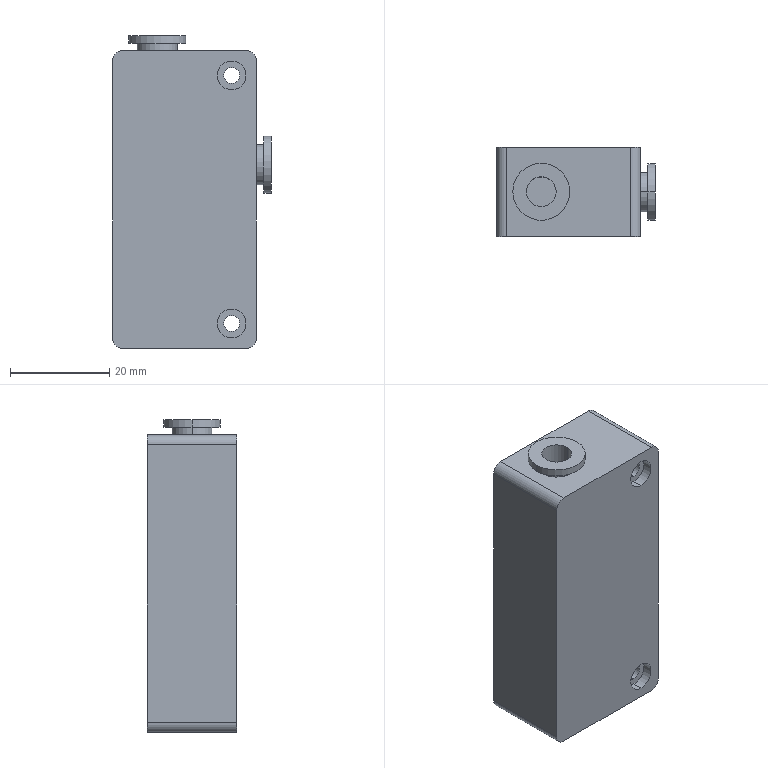Part | STEP file | ZH10BS_06_06_ZH10BS-06-06 | 1 solid | 44 faces | box 32 x 18 x 63 mm | volume 30323 mm3 | cylinder 28 | plane 16 | commonest cylinder face diameters 5.8 x8 3.2 x4 4 x4 6 x4 8 x4 11.5 x4
STEP:
#1=CARTESIAN_POINT('',(17.5,9.,10.));
#2=VERTEX_POINT('',#1);
#3=CARTESIAN_POINT('',(17.5,9.,4.));
#4=VERTEX_POINT('',#3);
#5=CARTESIAN_POINT('',(17.5,9.,7.));
#6=DIRECTION('',(1.,0.,0.));
#7=DIRECTION('',(0.,0.,1.));
#8=AXIS2_PLACEMENT_3D('',#5,#6,#7);
#9=CIRCLE('',#8,3.);
#10=EDGE_CURVE('',#2,#4,#9,.T.);
#11=ORIENTED_EDGE('',*,*,#10,.T.);
#12=CARTESIAN_POINT('',(0.5,9.,4.));
#13=VERTEX_POINT('',#12);
#14=CARTESIAN_POINT('',(17.51,9.,4.));
#15=DIRECTION('',(-1.,0.,0.));
#16=VECTOR('',#15,1000.);
#17=LINE('',#14,#16);
#18=EDGE_CURVE('',#4,#13,#17,.T.);
#19=ORIENTED_EDGE('',*,*,#18,.T.);
#20=CARTESIAN_POINT('',(0.5,9.,10.));
#21=VERTEX_POINT('',#20);
#22=CARTESIAN_POINT('',(0.5,9.,7.));
#23=DIRECTION('',(-1.,0.,0.));
#24=DIRECTION('',(0.,0.,1.));
#25=AXIS2_PLACEMENT_3D('',#22,#23,#24);
#26=CIRCLE('',#25,3.);
#27=EDGE_CURVE('',#13,#21,#26,.T.);
#28=ORIENTED_EDGE('',*,*,#27,.T.);
#29=CARTESIAN_POINT('',(17.51,9.,10.));
#30=DIRECTION('',(-1.,0.,0.));
#31=VECTOR('',#30,1000.);
#32=LINE('',#29,#31);
#33=EDGE_CURVE('',#2,#21,#32,.T.);
#34=ORIENTED_EDGE('',*,*,#33,.F.);
#35=EDGE_LOOP('',(#11,#19,#28,#34));
#36=FACE_OUTER_BOUND('',#35,.T.);
#37=CARTESIAN_POINT('',(17.51,9.,7.));
#38=DIRECTION('',(-1.,0.,0.));
#39=DIRECTION('',(0.,0.,1.));
#40=AXIS2_PLACEMENT_3D('',#37,#38,#39);
#41=CYLINDRICAL_SURFACE('',#40,3.);
#42=ADVANCED_FACE('',(#36),#41,.F.);
#43=CARTESIAN_POINT('',(16.,9.,1.25));
#44=VERTEX_POINT('',#43);
#45=CARTESIAN_POINT('',(16.,9.,12.75));
#46=VERTEX_POINT('',#45);
#47=CARTESIAN_POINT('',(16.,9.,7.));
#48=DIRECTION('',(1.,0.,0.));
#49=DIRECTION('',(0.,0.,-1.));
#50=AXIS2_PLACEMENT_3D('',#47,#48,#49);
#51=CIRCLE('',#50,5.75);
#52=EDGE_CURVE('',#44,#46,#51,.T.);
#53=ORIENTED_EDGE('',*,*,#52,.T.);
#54=CARTESIAN_POINT('',(17.5,9.,12.75));
#55=VERTEX_POINT('',#54);
#56=CARTESIAN_POINT('',(14.49,9.,12.75));
#57=DIRECTION('',(1.,0.,0.));
#58=VECTOR('',#57,1000.);
#59=LINE('',#56,#58);
#60=EDGE_CURVE('',#46,#55,#59,.T.);
#61=ORIENTED_EDGE('',*,*,#60,.T.);
#62=CARTESIAN_POINT('',(17.5,9.,1.25));
#63=VERTEX_POINT('',#62);
#64=CARTESIAN_POINT('',(17.5,9.,7.));
#65=DIRECTION('',(1.,0.,0.));
#66=DIRECTION('',(0.,0.,-1.));
#67=AXIS2_PLACEMENT_3D('',#64,#65,#66);
#68=CIRCLE('',#67,5.75);
#69=EDGE_CURVE('',#63,#55,#68,.T.);
#70=ORIENTED_EDGE('',*,*,#69,.F.);
#71=CARTESIAN_POINT('',(14.49,9.,1.25));
#72=DIRECTION('',(1.,0.,0.));
#73=VECTOR('',#72,1000.);
#74=LINE('',#71,#73);
#75=EDGE_CURVE('',#44,#63,#74,.T.);
#76=ORIENTED_EDGE('',*,*,#75,.F.);
#77=EDGE_LOOP('',(#53,#61,#70,#76));
#78=FACE_OUTER_BOUND('',#77,.T.);
#79=CARTESIAN_POINT('',(14.49,9.,7.));
#80=DIRECTION('',(1.,0.,0.));
#81=DIRECTION('',(0.,0.,-1.));
#82=AXIS2_PLACEMENT_3D('',#79,#80,#81);
#83=CYLINDRICAL_SURFACE('',#82,5.75);
#84=ADVANCED_FACE('',(#78),#83,.T.);
#85=CARTESIAN_POINT('',(14.5,9.,3.));
#86=VERTEX_POINT('',#85);
#87=CARTESIAN_POINT('',(14.5,9.,11.));
#88=VERTEX_POINT('',#87);
#89=CARTESIAN_POINT('',(14.5,9.,7.));
#90=DIRECTION('',(1.,0.,0.));
#91=DIRECTION('',(0.,0.,1.));
#92=AXIS2_PLACEMENT_3D('',#89,#90,#91);
#93=CIRCLE('',#92,4.);
#94=EDGE_CURVE('',#86,#88,#93,.T.);
#95=ORIENTED_EDGE('',*,*,#94,.T.);
#96=CARTESIAN_POINT('',(16.,9.,11.));
#97=VERTEX_POINT('',#96);
#98=CARTESIAN_POINT('',(14.49,9.,11.));
#99=DIRECTION('',(1.,0.,0.));
#100=VECTOR('',#99,1000.);
#101=LINE('',#98,#100);
#102=EDGE_CURVE('',#88,#97,#101,.T.);
#103=ORIENTED_EDGE('',*,*,#102,.T.);
#104=CARTESIAN_POINT('',(16.,9.,3.));
#105=VERTEX_POINT('',#104);
#106=CARTESIAN_POINT('',(16.,9.,7.));
#107=DIRECTION('',(1.,0.,0.));
#108=DIRECTION('',(0.,0.,-1.));
#109=AXIS2_PLACEMENT_3D('',#106,#107,#108);
#110=CIRCLE('',#109,4.);
#111=EDGE_CURVE('',#105,#97,#110,.T.);
#112=ORIENTED_EDGE('',*,*,#111,.F.);
#113=CARTESIAN_POINT('',(14.49,9.,3.));
#114=DIRECTION('',(1.,0.,0.));
#115=VECTOR('',#114,1000.);
#116=LINE('',#113,#115);
#117=EDGE_CURVE('',#86,#105,#116,.T.);
#118=ORIENTED_EDGE('',*,*,#117,.F.);
#119=EDGE_LOOP('',(#95,#103,#112,#118));
#120=FACE_OUTER_BOUND('',#119,.T.);
#121=CARTESIAN_POINT('',(14.49,9.,7.));
#122=DIRECTION('',(1.,0.,0.));
#123=DIRECTION('',(0.,0.,-1.));
#124=AXIS2_PLACEMENT_3D('',#121,#122,#123);
#125=CYLINDRICAL_SURFACE('',#124,4.);
#126=ADVANCED_FACE('',(#120),#125,.T.);
#127=CARTESIAN_POINT('',(-8.5,9.,16.));
#128=VERTEX_POINT('',#127);
#129=CARTESIAN_POINT('',(-2.5,9.,16.));
#130=VERTEX_POINT('',#129);
#131=CARTESIAN_POINT('',(-5.5,9.,16.));
#132=DIRECTION('',(0.,0.,1.));
#133=DIRECTION('',(1.,0.,0.));
#134=AXIS2_PLACEMENT_3D('',#131,#132,#133);
#135=CIRCLE('',#134,3.);
#136=EDGE_CURVE('',#128,#130,#135,.T.);
#137=ORIENTED_EDGE('',*,*,#136,.F.);
#138=CARTESIAN_POINT('',(-8.5,9.,33.));
#139=VERTEX_POINT('',#138);
#140=CARTESIAN_POINT('',(-8.5,9.,16.));
#141=DIRECTION('',(0.,0.,1.));
#142=VECTOR('',#141,1000.);
#143=LINE('',#140,#142);
#144=EDGE_CURVE('',#128,#139,#143,.T.);
#145=ORIENTED_EDGE('',*,*,#144,.T.);
#146=CARTESIAN_POINT('',(-2.5,9.,33.));
#147=VERTEX_POINT('',#146);
#148=CARTESIAN_POINT('',(-5.5,9.,33.));
#149=DIRECTION('',(0.,0.,1.));
#150=DIRECTION('',(-1.,0.,0.));
#151=AXIS2_PLACEMENT_3D('',#148,#149,#150);
#152=CIRCLE('',#151,3.);
#153=EDGE_CURVE('',#139,#147,#152,.T.);
#154=ORIENTED_EDGE('',*,*,#153,.T.);
#155=CARTESIAN_POINT('',(-2.5,9.,16.));
#156=DIRECTION('',(0.,0.,1.));
#157=VECTOR('',#156,1000.);
#158=LINE('',#155,#157);
#159=EDGE_CURVE('',#130,#147,#158,.T.);
#160=ORIENTED_EDGE('',*,*,#159,.F.);
#161=EDGE_LOOP('',(#137,#145,#154,#160));
#162=FACE_OUTER_BOUND('',#161,.T.);
#163=CARTESIAN_POINT('',(-5.5,9.,16.));
#164=DIRECTION('',(0.,0.,1.));
#165=DIRECTION('',(1.,0.,0.));
#166=AXIS2_PLACEMENT_3D('',#163,#164,#165);
#167=CYLINDRICAL_SURFACE('',#166,3.);
#168=ADVANCED_FACE('',(#162),#167,.F.);
#169=CARTESIAN_POINT('',(0.25,9.,31.5));
#170=VERTEX_POINT('',#169);
#171=CARTESIAN_POINT('',(-11.25,9.,31.5));
#172=VERTEX_POINT('',#171);
#173=CARTESIAN_POINT('',(-5.5,9.,31.5));
#174=DIRECTION('',(0.,0.,1.));
#175=DIRECTION('',(1.,0.,0.));
#176=AXIS2_PLACEMENT_3D('',#173,#174,#175);
#177=CIRCLE('',#176,5.75);
#178=EDGE_CURVE('',#170,#172,#177,.T.);
#179=ORIENTED_EDGE('',*,*,#178,.T.);
#180=CARTESIAN_POINT('',(-11.25,9.,33.));
#181=VERTEX_POINT('',#180);
#182=CARTESIAN_POINT('',(-11.25,9.,29.99));
#183=DIRECTION('',(0.,0.,1.));
#184=VECTOR('',#183,1000.);
#185=LINE('',#182,#184);
#186=EDGE_CURVE('',#172,#181,#185,.T.);
#187=ORIENTED_EDGE('',*,*,#186,.T.);
#188=CARTESIAN_POINT('',(0.25,9.,33.));
#189=VERTEX_POINT('',#188);
#190=CARTESIAN_POINT('',(-5.5,9.,33.));
#191=DIRECTION('',(0.,0.,1.));
#192=DIRECTION('',(1.,0.,0.));
#193=AXIS2_PLACEMENT_3D('',#190,#191,#192);
#194=CIRCLE('',#193,5.75);
#195=EDGE_CURVE('',#189,#181,#194,.T.);
#196=ORIENTED_EDGE('',*,*,#195,.F.);
#197=CARTESIAN_POINT('',(0.25,9.,29.99));
#198=DIRECTION('',(0.,0.,1.));
#199=VECTOR('',#198,1000.);
#200=LINE('',#197,#199);
#201=EDGE_CURVE('',#170,#189,#200,.T.);
#202=ORIENTED_EDGE('',*,*,#201,.F.);
#203=EDGE_LOOP('',(#179,#187,#196,#202));
#204=FACE_OUTER_BOUND('',#203,.T.);
#205=CARTESIAN_POINT('',(-5.5,9.,29.99));
#206=DIRECTION('',(0.,0.,1.));
#207=DIRECTION('',(1.,0.,0.));
#208=AXIS2_PLACEMENT_3D('',#205,#206,#207);
#209=CYLINDRICAL_SURFACE('',#208,5.75);
#210=ADVANCED_FACE('',(#204),#209,.T.);
#211=CARTESIAN_POINT('',(-1.5,9.,30.));
#212=VERTEX_POINT('',#211);
#213=CARTESIAN_POINT('',(-9.5,9.,30.));
#214=VERTEX_POINT('',#213);
#215=CARTESIAN_POINT('',(-5.5,9.,30.));
#216=DIRECTION('',(0.,0.,1.));
#217=DIRECTION('',(-1.,0.,0.));
#218=AXIS2_PLACEMENT_3D('',#215,#216,#217);
#219=CIRCLE('',#218,4.);
#220=EDGE_CURVE('',#212,#214,#219,.T.);
#221=ORIENTED_EDGE('',*,*,#220,.T.);
#222=CARTESIAN_POINT('',(-9.5,9.,31.5));
#223=VERTEX_POINT('',#222);
#224=CARTESIAN_POINT('',(-9.5,9.,29.99));
#225=DIRECTION('',(0.,0.,1.));
#226=VECTOR('',#225,1000.);
#227=LINE('',#224,#226);
#228=EDGE_CURVE('',#214,#223,#227,.T.);
#229=ORIENTED_EDGE('',*,*,#228,.T.);
#230=CARTESIAN_POINT('',(-1.5,9.,31.5));
#231=VERTEX_POINT('',#230);
#232=CARTESIAN_POINT('',(-5.5,9.,31.5));
#233=DIRECTION('',(0.,0.,1.));
#234=DIRECTION('',(1.,0.,0.));
#235=AXIS2_PLACEMENT_3D('',#232,#233,#234);
#236=CIRCLE('',#235,4.);
#237=EDGE_CURVE('',#231,#223,#236,.T.);
#238=ORIENTED_EDGE('',*,*,#237,.F.);
#239=CARTESIAN_POINT('',(-1.5,9.,29.99));
#240=DIRECTION('',(0.,0.,1.));
#241=VECTOR('',#240,1000.);
#242=LINE('',#239,#241);
#243=EDGE_CURVE('',#212,#231,#242,.T.);
#244=ORIENTED_EDGE('',*,*,#243,.F.);
#245=EDGE_LOOP('',(#221,#229,#238,#244));
#246=FACE_OUTER_BOUND('',#245,.T.);
#247=CARTESIAN_POINT('',(-5.5,9.,29.99));
#248=DIRECTION('',(0.,0.,1.));
#249=DIRECTION('',(1.,0.,0.));
#250=AXIS2_PLACEMENT_3D('',#247,#248,#249);
#251=CYLINDRICAL_SURFACE('',#250,4.);
#252=ADVANCED_FACE('',(#246),#251,.T.);
#253=CARTESIAN_POINT('',(9.5,2.,-26.6));
#254=VERTEX_POINT('',#253);
#255=CARTESIAN_POINT('',(9.5,2.,-23.4));
#256=VERTEX_POINT('',#255);
#257=CARTESIAN_POINT('',(9.5,2.,-25.));
#258=DIRECTION('',(0.,1.,0.));
#259=DIRECTION('',(0.,0.,1.));
#260=AXIS2_PLACEMENT_3D('',#257,#258,#259);
#261=CIRCLE('',#260,1.6);
#262=EDGE_CURVE('',#254,#256,#261,.T.);
#263=ORIENTED_EDGE('',*,*,#262,.F.);
#264=CARTESIAN_POINT('',(9.5,16.,-26.6));
#265=VERTEX_POINT('',#264);
#266=CARTESIAN_POINT('',(9.5,-2.,-26.6));
#267=DIRECTION('',(0.,1.,0.));
#268=VECTOR('',#267,1000.);
#269=LINE('',#266,#268);
#270=EDGE_CURVE('',#254,#265,#269,.T.);
#271=ORIENTED_EDGE('',*,*,#270,.T.);
#272=CARTESIAN_POINT('',(9.5,16.,-23.4));
#273=VERTEX_POINT('',#272);
#274=CARTESIAN_POINT('',(9.5,16.,-25.));
#275=DIRECTION('',(0.,1.,0.));
#276=DIRECTION('',(0.,0.,1.));
#277=AXIS2_PLACEMENT_3D('',#274,#275,#276);
#278=CIRCLE('',#277,1.6);
#279=EDGE_CURVE('',#265,#273,#278,.T.);
#280=ORIENTED_EDGE('',*,*,#279,.T.);
#281=CARTESIAN_POINT('',(9.5,-2.,-23.4));
#282=DIRECTION('',(0.,1.,0.));
#283=VECTOR('',#282,1000.);
#284=LINE('',#281,#283);
#285=EDGE_CURVE('',#256,#273,#284,.T.);
#286=ORIENTED_EDGE('',*,*,#285,.F.);
#287=EDGE_LOOP('',(#263,#271,#280,#286));
#288=FACE_OUTER_BOUND('',#287,.T.);
#289=CARTESIAN_POINT('',(9.5,-2.,-25.));
#290=DIRECTION('',(0.,1.,0.));
#291=DIRECTION('',(0.,0.,1.));
#292=AXIS2_PLACEMENT_3D('',#289,#290,#291);
#293=CYLINDRICAL_SURFACE('',#292,1.6);
#294=ADVANCED_FACE('',(#288),#293,.F.);
#295=CARTESIAN_POINT('',(9.5,16.,-27.9));
#296=VERTEX_POINT('',#295);
#297=CARTESIAN_POINT('',(9.5,16.,-22.1));
#298=VERTEX_POINT('',#297);
#299=CARTESIAN_POINT('',(9.5,16.,-25.));
#300=DIRECTION('',(0.,1.,0.));
#301=DIRECTION('',(0.,0.,1.));
#302=AXIS2_PLACEMENT_3D('',#299,#300,#301);
#303=CIRCLE('',#302,2.9);
#304=EDGE_CURVE('',#296,#298,#303,.T.);
#305=ORIENTED_EDGE('',*,*,#304,.F.);
#306=CARTESIAN_POINT('',(9.5,18.,-27.9));
#307=VERTEX_POINT('',#306);
#308=CARTESIAN_POINT('',(9.5,-2.,-27.9));
#309=DIRECTION('',(0.,1.,0.));
#310=VECTOR('',#309,1000.);
#311=LINE('',#308,#310);
#312=EDGE_CURVE('',#296,#307,#311,.T.);
#313=ORIENTED_EDGE('',*,*,#312,.T.);
#314=CARTESIAN_POINT('',(9.5,18.,-22.1));
#315=VERTEX_POINT('',#314);
#316=CARTESIAN_POINT('',(9.5,18.,-25.));
#317=DIRECTION('',(0.,-1.,0.));
#318=DIRECTION('',(0.,0.,1.));
#319=AXIS2_PLACEMENT_3D('',#316,#317,#318);
#320=CIRCLE('',#319,2.9);
#321=EDGE_CURVE('',#315,#307,#320,.T.);
#322=ORIENTED_EDGE('',*,*,#321,.F.);
#323=CARTESIAN_POINT('',(9.5,-2.,-22.1));
#324=DIRECTION('',(0.,1.,0.));
#325=VECTOR('',#324,1000.);
#326=LINE('',#323,#325);
#327=EDGE_CURVE('',#298,#315,#326,.T.);
#328=ORIENTED_EDGE('',*,*,#327,.F.);
#329=EDGE_LOOP('',(#305,#313,#322,#328));
#330=FACE_OUTER_BOUND('',#329,.T.);
#331=CARTESIAN_POINT('',(9.5,-2.,-25.));
#332=DIRECTION('',(0.,1.,0.));
#333=DIRECTION('',(0.,0.,1.));
#334=AXIS2_PLACEMENT_3D('',#331,#332,#333);
#335=CYLINDRICAL_SURFACE('',#334,2.9);
#336=ADVANCED_FACE('',(#330),#335,.F.);
#337=CARTESIAN_POINT('',(9.5,0.,-22.1));
#338=VERTEX_POINT('',#337);
#339=CARTESIAN_POINT('',(9.5,0.,-27.9));
#340=VERTEX_POINT('',#339);
#341=CARTESIAN_POINT('',(9.5,0.,-25.));
#342=DIRECTION('',(0.,-1.,0.));
#343=DIRECTION('',(0.,0.,1.));
#344=AXIS2_PLACEMENT_3D('',#341,#342,#343);
#345=CIRCLE('',#344,2.9);
#346=EDGE_CURVE('',#338,#340,#345,.T.);
#347=ORIENTED_EDGE('',*,*,#346,.T.);
#348=CARTESIAN_POINT('',(9.5,2.,-27.9));
#349=VERTEX_POINT('',#348);
#350=CARTESIAN_POINT('',(9.5,-2.,-27.9));
#351=DIRECTION('',(0.,1.,0.));
#352=VECTOR('',#351,1000.);
#353=LINE('',#350,#352);
#354=EDGE_CURVE('',#340,#349,#353,.T.);
#355=ORIENTED_EDGE('',*,*,#354,.T.);
#356=CARTESIAN_POINT('',(9.5,2.,-22.1));
#357=VERTEX_POINT('',#356);
#358=CARTESIAN_POINT('',(9.5,2.,-25.));
#359=DIRECTION('',(0.,1.,0.));
#360=DIRECTION('',(0.,0.,1.));
#361=AXIS2_PLACEMENT_3D('',#358,#359,#360);
#362=CIRCLE('',#361,2.9);
#363=EDGE_CURVE('',#349,#357,#362,.T.);
#364=ORIENTED_EDGE('',*,*,#363,.T.);
#365=CARTESIAN_POINT('',(9.5,-2.,-22.1));
#366=DIRECTION('',(0.,1.,0.));
#367=VECTOR('',#366,1000.);
#368=LINE('',#365,#367);
#369=EDGE_CURVE('',#338,#357,#368,.T.);
#370=ORIENTED_EDGE('',*,*,#369,.F.);
#371=EDGE_LOOP('',(#347,#355,#364,#370));
#372=FACE_OUTER_BOUND('',#371,.T.);
#373=CARTESIAN_POINT('',(9.5,-2.,-25.));
#374=DIRECTION('',(0.,1.,0.));
#375=DIRECTION('',(0.,0.,1.));
#376=AXIS2_PLACEMENT_3D('',#373,#374,#375);
#377=CYLINDRICAL_SURFACE('',#376,2.9);
#378=ADVANCED_FACE('',(#372),#377,.F.);
#379=CARTESIAN_POINT('',(9.5,2.,23.4));
#380=VERTEX_POINT('',#379);
#381=CARTESIAN_POINT('',(9.5,2.,26.6));
#382=VERTEX_POINT('',#381);
#383=CARTESIAN_POINT('',(9.5,2.,25.));
#384=DIRECTION('',(0.,1.,0.));
#385=DIRECTION('',(0.,0.,1.));
#386=AXIS2_PLACEMENT_3D('',#383,#384,#385);
#387=CIRCLE('',#386,1.6);
#388=EDGE_CURVE('',#380,#382,#387,.T.);
#389=ORIENTED_EDGE('',*,*,#388,.F.);
#390=CARTESIAN_POINT('',(9.5,16.,23.4));
#391=VERTEX_POINT('',#390);
#392=CARTESIAN_POINT('',(9.5,-2.,23.4));
#393=DIRECTION('',(0.,1.,0.));
#394=VECTOR('',#393,1000.);
#395=LINE('',#392,#394);
#396=EDGE_CURVE('',#380,#391,#395,.T.);
#397=ORIENTED_EDGE('',*,*,#396,.T.);
#398=CARTESIAN_POINT('',(9.5,16.,26.6));
#399=VERTEX_POINT('',#398);
#400=CARTESIAN_POINT('',(9.5,16.,25.));
#401=DIRECTION('',(0.,1.,0.));
#402=DIRECTION('',(0.,0.,1.));
#403=AXIS2_PLACEMENT_3D('',#400,#401,#402);
#404=CIRCLE('',#403,1.6);
#405=EDGE_CURVE('',#391,#399,#404,.T.);
#406=ORIENTED_EDGE('',*,*,#405,.T.);
#407=CARTESIAN_POINT('',(9.5,-2.,26.6));
#408=DIRECTION('',(0.,1.,0.));
#409=VECTOR('',#408,1000.);
#410=LINE('',#407,#409);
#411=EDGE_CURVE('',#382,#399,#410,.T.);
#412=ORIENTED_EDGE('',*,*,#411,.F.);
#413=EDGE_LOOP('',(#389,#397,#406,#412));
#414=FACE_OUTER_BOUND('',#413,.T.);
#415=CARTESIAN_POINT('',(9.5,-2.,25.));
#416=DIRECTION('',(0.,1.,0.));
#417=DIRECTION('',(0.,0.,1.));
#418=AXIS2_PLACEMENT_3D('',#415,#416,#417);
#419=CYLINDRICAL_SURFACE('',#418,1.6);
#420=ADVANCED_FACE('',(#414),#419,.F.);
#421=CARTESIAN_POINT('',(9.5,16.,22.1));
#422=VERTEX_POINT('',#421);
#423=CARTESIAN_POINT('',(9.5,16.,27.9));
#424=VERTEX_POINT('',#423);
#425=CARTESIAN_POINT('',(9.5,16.,25.));
#426=DIRECTION('',(0.,1.,0.));
#427=DIRECTION('',(0.,0.,1.));
#428=AXIS2_PLACEMENT_3D('',#425,#426,#427);
#429=CIRCLE('',#428,2.9);
#430=EDGE_CURVE('',#422,#424,#429,.T.);
#431=ORIENTED_EDGE('',*,*,#430,.F.);
#432=CARTESIAN_POINT('',(9.5,18.,22.1));
#433=VERTEX_POINT('',#432);
#434=CARTESIAN_POINT('',(9.5,-2.,22.1));
#435=DIRECTION('',(0.,1.,0.));
#436=VECTOR('',#435,1000.);
#437=LINE('',#434,#436);
#438=EDGE_CURVE('',#422,#433,#437,.T.);
#439=ORIENTED_EDGE('',*,*,#438,.T.);
#440=CARTESIAN_POINT('',(9.5,18.,27.9));
#441=VERTEX_POINT('',#440);
#442=CARTESIAN_POINT('',(9.5,18.,25.));
#443=DIRECTION('',(0.,-1.,0.));
#444=DIRECTION('',(0.,0.,1.));
#445=AXIS2_PLACEMENT_3D('',#442,#443,#444);
#446=CIRCLE('',#445,2.9);
#447=EDGE_CURVE('',#441,#433,#446,.T.);
#448=ORIENTED_EDGE('',*,*,#447,.F.);
#449=CARTESIAN_POINT('',(9.5,-2.,27.9));
#450=DIRECTION('',(0.,1.,0.));
#451=VECTOR('',#450,1000.);
#452=LINE('',#449,#451);
#453=EDGE_CURVE('',#424,#441,#452,.T.);
#454=ORIENTED_EDGE('',*,*,#453,.F.);
#455=EDGE_LOOP('',(#431,#439,#448,#454));
#456=FACE_OUTER_BOUND('',#455,.T.);
#457=CARTESIAN_POINT('',(9.5,-2.,25.));
#458=DIRECTION('',(0.,1.,0.));
#459=DIRECTION('',(0.,0.,1.));
#460=AXIS2_PLACEMENT_3D('',#457,#458,#459);
#461=CYLINDRICAL_SURFACE('',#460,2.9);
#462=ADVANCED_FACE('',(#456),#461,.F.);
#463=CARTESIAN_POINT('',(9.5,0.,27.9));
#464=VERTEX_POINT('',#463);
#465=CARTESIAN_POINT('',(9.5,0.,22.1));
#466=VERTEX_POINT('',#465);
#467=CARTESIAN_POINT('',(9.5,0.,25.));
#468=DIRECTION('',(0.,-1.,0.));
#469=DIRECTION('',(0.,0.,1.));
#470=AXIS2_PLACEMENT_3D('',#467,#468,#469);
#471=CIRCLE('',#470,2.9);
#472=EDGE_CURVE('',#464,#466,#471,.T.);
#473=ORIENTED_EDGE('',*,*,#472,.T.);
#474=CARTESIAN_POINT('',(9.5,2.,22.1));
#475=VERTEX_POINT('',#474);
#476=CARTESIAN_POINT('',(9.5,-2.,22.1));
#477=DIRECTION('',(0.,1.,0.));
#478=VECTOR('',#477,1000.);
#479=LINE('',#476,#478);
#480=EDGE_CURVE('',#466,#475,#479,.T.);
#481=ORIENTED_EDGE('',*,*,#480,.T.);
#482=CARTESIAN_POINT('',(9.5,2.,27.9));
#483=VERTEX_POINT('',#482);
#484=CARTESIAN_POINT('',(9.5,2.,25.));
#485=DIRECTION('',(0.,1.,0.));
#486=DIRECTION('',(0.,0.,1.));
#487=AXIS2_PLACEMENT_3D('',#484,#485,#486);
#488=CIRCLE('',#487,2.9);
#489=EDGE_CURVE('',#475,#483,#488,.T.);
#490=ORIENTED_EDGE('',*,*,#489,.T.);
#491=CARTESIAN_POINT('',(9.5,-2.,27.9));
#492=DIRECTION('',(0.,1.,0.));
#493=VECTOR('',#492,1000.);
#494=LINE('',#491,#493);
#495=EDGE_CURVE('',#464,#483,#494,.T.);
#496=ORIENTED_EDGE('',*,*,#495,.F.);
#497=EDGE_LOOP('',(#473,#481,#490,#496));
#498=FACE_OUTER_BOUND('',#497,.T.);
#499=CARTESIAN_POINT('',(9.5,-2.,25.));
#500=DIRECTION('',(0.,1.,0.));
#501=DIRECTION('',(0.,0.,1.));
#502=AXIS2_PLACEMENT_3D('',#499,#500,#501);
#503=CYLINDRICAL_SURFACE('',#502,2.9);
#504=ADVANCED_FACE('',(#498),#503,.F.);
#505=ORIENTED_EDGE('',*,*,#69,.T.);
#506=CARTESIAN_POINT('',(17.5,9.,7.));
#507=DIRECTION('',(1.,0.,0.));
#508=DIRECTION('',(0.,0.,-1.));
#509=AXIS2_PLACEMENT_3D('',#506,#507,#508);
#510=CIRCLE('',#509,5.75);
#511=EDGE_CURVE('',#55,#63,#510,.T.);
#512=ORIENTED_EDGE('',*,*,#511,.T.);
#513=EDGE_LOOP('',(#505,#512));
#514=FACE_OUTER_BOUND('',#513,.T.);
#515=ORIENTED_EDGE('',*,*,#10,.F.);
#516=CARTESIAN_POINT('',(17.5,9.,7.));
#517=DIRECTION('',(1.,0.,0.));
#518=DIRECTION('',(0.,0.,1.));
#519=AXIS2_PLACEMENT_3D('',#516,#517,#518);
#520=CIRCLE('',#519,3.);
#521=EDGE_CURVE('',#4,#2,#520,.T.);
#522=ORIENTED_EDGE('',*,*,#521,.F.);
#523=EDGE_LOOP('',(#515,#522));
#524=FACE_BOUND('',#523,.T.);
#525=CARTESIAN_POINT('',(17.5,9.,7.));
#526=DIRECTION('',(-1.,0.,0.));
#527=DIRECTION('',(0.,0.,1.));
#528=AXIS2_PLACEMENT_3D('',#525,#526,#527);
#529=PLANE('',#528);
#530=ADVANCED_FACE('',(#514,#524),#529,.F.);
#531=CARTESIAN_POINT('',(14.5,0.,28.));
#532=VERTEX_POINT('',#531);
#533=CARTESIAN_POINT('',(14.5,0.,-28.));
#534=VERTEX_POINT('',#533);
#535=CARTESIAN_POINT('',(14.5,0.,28.));
#536=DIRECTION('',(0.,0.,-1.));
#537=VECTOR('',#536,1000.);
#538=LINE('',#535,#537);
#539=EDGE_CURVE('',#532,#534,#538,.T.);
#540=ORIENTED_EDGE('',*,*,#539,.T.);
#541=CARTESIAN_POINT('',(14.5,18.,-28.));
#542=VERTEX_POINT('',#541);
#543=CARTESIAN_POINT('',(14.5,18.,-28.));
#544=DIRECTION('',(0.,-1.,0.));
#545=VECTOR('',#544,1000.);
#546=LINE('',#543,#545);
#547=EDGE_CURVE('',#542,#534,#546,.T.);
#548=ORIENTED_EDGE('',*,*,#547,.F.);
#549=CARTESIAN_POINT('',(14.5,18.,28.));
#550=VERTEX_POINT('',#549);
#551=CARTESIAN_POINT('',(14.5,18.,28.));
#552=DIRECTION('',(0.,0.,-1.));
#553=VECTOR('',#552,1000.);
#554=LINE('',#551,#553);
#555=EDGE_CURVE('',#550,#542,#554,.T.);
#556=ORIENTED_EDGE('',*,*,#555,.F.);
#557=CARTESIAN_POINT('',(14.5,18.,28.));
#558=DIRECTION('',(0.,-1.,0.));
#559=VECTOR('',#558,1000.);
#560=LINE('',#557,#559);
#561=EDGE_CURVE('',#550,#532,#560,.T.);
#562=ORIENTED_EDGE('',*,*,#561,.T.);
#563=EDGE_LOOP('',(#540,#548,#556,#562));
#564=FACE_OUTER_BOUND('',#563,.T.);
#565=ORIENTED_EDGE('',*,*,#94,.F.);
#566=CARTESIAN_POINT('',(14.5,9.,7.));
#567=DIRECTION('',(1.,0.,0.));
#568=DIRECTION('',(0.,0.,1.));
#569=AXIS2_PLACEMENT_3D('',#566,#567,#568);
#570=CIRCLE('',#569,4.);
#571=EDGE_CURVE('',#88,#86,#570,.T.);
#572=ORIENTED_EDGE('',*,*,#571,.F.);
#573=EDGE_LOOP('',(#565,#572));
#574=FACE_BOUND('',#573,.T.);
#575=CARTESIAN_POINT('',(14.5,18.,28.));
#576=DIRECTION('',(-1.,0.,0.));
#577=DIRECTION('',(0.,0.,1.));
#578=AXIS2_PLACEMENT_3D('',#575,#576,#577);
#579=PLANE('',#578);
#580=ADVANCED_FACE('',(#564,#574),#579,.F.);
#581=ORIENTED_EDGE('',*,*,#195,.T.);
#582=CARTESIAN_POINT('',(-5.5,9.,33.));
#583=DIRECTION('',(0.,0.,1.));
#584=DIRECTION('',(1.,0.,0.));
#585=AXIS2_PLACEMENT_3D('',#582,#583,#584);
#586=CIRCLE('',#585,5.75);
#587=EDGE_CURVE('',#181,#189,#586,.T.);
#588=ORIENTED_EDGE('',*,*,#587,.T.);
#589=EDGE_LOOP('',(#581,#588));
#590=FACE_OUTER_BOUND('',#589,.T.);
#591=CARTESIAN_POINT('',(-5.5,9.,33.));
#592=DIRECTION('',(0.,0.,1.));
#593=DIRECTION('',(-1.,0.,0.));
#594=AXIS2_PLACEMENT_3D('',#591,#592,#593);
#595=CIRCLE('',#594,3.);
#596=EDGE_CURVE('',#147,#139,#595,.T.);
#597=ORIENTED_EDGE('',*,*,#596,.F.);
#598=ORIENTED_EDGE('',*,*,#153,.F.);
#599=EDGE_LOOP('',(#597,#598));
#600=FACE_BOUND('',#599,.T.);
#601=CARTESIAN_POINT('',(-5.5,9.,33.));
#602=DIRECTION('',(0.,0.,-1.));
#603=DIRECTION('',(-1.,0.,0.));
#604=AXIS2_PLACEMENT_3D('',#601,#602,#603);
#605=PLANE('',#604);
#606=ADVANCED_FACE('',(#590,#600),#605,.F.);
#607=CARTESIAN_POINT('',(-12.5,0.,30.));
#608=VERTEX_POINT('',#607);
#609=CARTESIAN_POINT('',(12.5,0.,30.));
#610=VERTEX_POINT('',#609);
#611=CARTESIAN_POINT('',(-12.5,0.,30.));
#612=DIRECTION('',(1.,0.,0.));
#613=VECTOR('',#612,1000.);
#614=LINE('',#611,#613);
#615=EDGE_CURVE('',#608,#610,#614,.T.);
#616=ORIENTED_EDGE('',*,*,#615,.T.);
#617=CARTESIAN_POINT('',(12.5,18.,30.));
#618=VERTEX_POINT('',#617);
#619=CARTESIAN_POINT('',(12.5,18.,30.));
#620=DIRECTION('',(0.,-1.,0.));
#621=VECTOR('',#620,1000.);
#622=LINE('',#619,#621);
#623=EDGE_CURVE('',#618,#610,#622,.T.);
#624=ORIENTED_EDGE('',*,*,#623,.F.);
#625=CARTESIAN_POINT('',(-12.5,18.,30.));
#626=VERTEX_POINT('',#625);
#627=CARTESIAN_POINT('',(-12.5,18.,30.));
#628=DIRECTION('',(1.,0.,0.));
#629=VECTOR('',#628,1000.);
#630=LINE('',#627,#629);
#631=EDGE_CURVE('',#626,#618,#630,.T.);
#632=ORIENTED_EDGE('',*,*,#631,.F.);
#633=CARTESIAN_POINT('',(-12.5,18.,30.));
#634=DIRECTION('',(0.,-1.,0.));
#635=VECTOR('',#634,1000.);
#636=LINE('',#633,#635);
#637=EDGE_CURVE('',#626,#608,#636,.T.);
#638=ORIENTED_EDGE('',*,*,#637,.T.);
#639=EDGE_LOOP('',(#616,#624,#632,#638));
#640=FACE_OUTER_BOUND('',#639,.T.);
#641=ORIENTED_EDGE('',*,*,#220,.F.);
#642=CARTESIAN_POINT('',(-5.5,9.,30.));
#643=DIRECTION('',(0.,0.,1.));
#644=DIRECTION('',(-1.,0.,0.));
#645=AXIS2_PLACEMENT_3D('',#642,#643,#644);
#646=CIRCLE('',#645,4.);
#647=EDGE_CURVE('',#214,#212,#646,.T.);
#648=ORIENTED_EDGE('',*,*,#647,.F.);
#649=EDGE_LOOP('',(#641,#648));
#650=FACE_BOUND('',#649,.T.);
#651=CARTESIAN_POINT('',(-12.5,18.,30.));
#652=DIRECTION('',(0.,0.,-1.));
#653=DIRECTION('',(-1.,0.,0.));
#654=AXIS2_PLACEMENT_3D('',#651,#652,#653);
#655=PLANE('',#654);
#656=ADVANCED_FACE('',(#640,#650),#655,.F.);
#657=ORIENTED_EDGE('',*,*,#447,.T.);
#658=CARTESIAN_POINT('',(9.5,18.,25.));
#659=DIRECTION('',(0.,-1.,0.));
#660=DIRECTION('',(0.,0.,1.));
#661=AXIS2_PLACEMENT_3D('',#658,#659,#660);
#662=CIRCLE('',#661,2.9);
#663=EDGE_CURVE('',#433,#441,#662,.T.);
#664=ORIENTED_EDGE('',*,*,#663,.T.);
#665=EDGE_LOOP('',(#657,#664));
#666=FACE_BOUND('',#665,.T.);
#667=CARTESIAN_POINT('',(-14.5,18.,28.));
#668=VERTEX_POINT('',#667);
#669=CARTESIAN_POINT('',(-12.5,18.,28.));
#670=DIRECTION('',(0.,1.,0.));
#671=DIRECTION('',(0.,0.,1.));
#672=AXIS2_PLACEMENT_3D('',#669,#670,#671);
#673=CIRCLE('',#672,2.);
#674=EDGE_CURVE('',#668,#626,#673,.T.);
#675=ORIENTED_EDGE('',*,*,#674,.T.);
#676=ORIENTED_EDGE('',*,*,#631,.T.);
#677=CARTESIAN_POINT('',(12.5,18.,28.));
#678=DIRECTION('',(0.,1.,0.));
#679=DIRECTION('',(0.,0.,1.));
#680=AXIS2_PLACEMENT_3D('',#677,#678,#679);
#681=CIRCLE('',#680,2.);
#682=EDGE_CURVE('',#618,#550,#681,.T.);
#683=ORIENTED_EDGE('',*,*,#682,.T.);
#684=ORIENTED_EDGE('',*,*,#555,.T.);
#685=CARTESIAN_POINT('',(12.5,18.,-30.));
#686=VERTEX_POINT('',#685);
#687=CARTESIAN_POINT('',(12.5,18.,-28.));
#688=DIRECTION('',(0.,1.,0.));
#689=DIRECTION('',(0.,0.,1.));
#690=AXIS2_PLACEMENT_3D('',#687,#688,#689);
#691=CIRCLE('',#690,2.);
#692=EDGE_CURVE('',#542,#686,#691,.T.);
#693=ORIENTED_EDGE('',*,*,#692,.T.);
#694=CARTESIAN_POINT('',(-12.5,18.,-30.));
#695=VERTEX_POINT('',#694);
#696=CARTESIAN_POINT('',(12.5,18.,-30.));
#697=DIRECTION('',(-1.,0.,0.));
#698=VECTOR('',#697,1000.);
#699=LINE('',#696,#698);
#700=EDGE_CURVE('',#686,#695,#699,.T.);
#701=ORIENTED_EDGE('',*,*,#700,.T.);
#702=CARTESIAN_POINT('',(-14.5,18.,-28.));
#703=VERTEX_POINT('',#702);
#704=CARTESIAN_POINT('',(-12.5,18.,-28.));
#705=DIRECTION('',(0.,1.,0.));
#706=DIRECTION('',(0.,0.,1.));
#707=AXIS2_PLACEMENT_3D('',#704,#705,#706);
#708=CIRCLE('',#707,2.);
#709=EDGE_CURVE('',#695,#703,#708,.T.);
#710=ORIENTED_EDGE('',*,*,#709,.T.);
#711=CARTESIAN_POINT('',(-14.5,18.,-28.));
#712=DIRECTION('',(0.,0.,1.));
#713=VECTOR('',#712,1000.);
#714=LINE('',#711,#713);
#715=EDGE_CURVE('',#703,#668,#714,.T.);
#716=ORIENTED_EDGE('',*,*,#715,.T.);
#717=EDGE_LOOP('',(#675,#676,#683,#684,#693,#701,#710,#716));
#718=FACE_OUTER_BOUND('',#717,.T.);
#719=ORIENTED_EDGE('',*,*,#321,.T.);
#720=CARTESIAN_POINT('',(9.5,18.,-25.));
#721=DIRECTION('',(0.,-1.,0.));
#722=DIRECTION('',(0.,0.,1.));
#723=AXIS2_PLACEMENT_3D('',#720,#721,#722);
#724=CIRCLE('',#723,2.9);
#725=EDGE_CURVE('',#307,#315,#724,.T.);
#726=ORIENTED_EDGE('',*,*,#725,.T.);
#727=EDGE_LOOP('',(#719,#726));
#728=FACE_BOUND('',#727,.T.);
#729=CARTESIAN_POINT('',(-12.5,18.,28.));
#730=DIRECTION('',(0.,1.,0.));
#731=DIRECTION('',(0.,0.,1.));
#732=AXIS2_PLACEMENT_3D('',#729,#730,#731);
#733=PLANE('',#732);
#734=ADVANCED_FACE('',(#666,#718,#728),#733,.T.);
#735=ORIENTED_EDGE('',*,*,#472,.F.);
#736=CARTESIAN_POINT('',(9.5,0.,25.));
#737=DIRECTION('',(0.,-1.,0.));
#738=DIRECTION('',(0.,0.,1.));
#739=AXIS2_PLACEMENT_3D('',#736,#737,#738);
#740=CIRCLE('',#739,2.9);
#741=EDGE_CURVE('',#466,#464,#740,.T.);
#742=ORIENTED_EDGE('',*,*,#741,.F.);
#743=EDGE_LOOP('',(#735,#742));
#744=FACE_BOUND('',#743,.T.);
#745=CARTESIAN_POINT('',(-14.5,0.,28.));
#746=VERTEX_POINT('',#745);
#747=CARTESIAN_POINT('',(-12.5,0.,28.));
#748=DIRECTION('',(0.,1.,0.));
#749=DIRECTION('',(0.,0.,1.));
#750=AXIS2_PLACEMENT_3D('',#747,#748,#749);
#751=CIRCLE('',#750,2.);
#752=EDGE_CURVE('',#746,#608,#751,.T.);
#753=ORIENTED_EDGE('',*,*,#752,.F.);
#754=CARTESIAN_POINT('',(-14.5,0.,-28.));
#755=VERTEX_POINT('',#754);
#756=CARTESIAN_POINT('',(-14.5,0.,-28.));
#757=DIRECTION('',(0.,0.,1.));
#758=VECTOR('',#757,1000.);
#759=LINE('',#756,#758);
#760=EDGE_CURVE('',#755,#746,#759,.T.);
#761=ORIENTED_EDGE('',*,*,#760,.F.);
#762=CARTESIAN_POINT('',(-12.5,0.,-30.));
#763=VERTEX_POINT('',#762);
#764=CARTESIAN_POINT('',(-12.5,0.,-28.));
#765=DIRECTION('',(0.,1.,0.));
#766=DIRECTION('',(0.,0.,1.));
#767=AXIS2_PLACEMENT_3D('',#764,#765,#766);
#768=CIRCLE('',#767,2.);
#769=EDGE_CURVE('',#763,#755,#768,.T.);
#770=ORIENTED_EDGE('',*,*,#769,.F.);
#771=CARTESIAN_POINT('',(12.5,0.,-30.));
#772=VERTEX_POINT('',#771);
#773=CARTESIAN_POINT('',(12.5,0.,-30.));
#774=DIRECTION('',(-1.,0.,0.));
#775=VECTOR('',#774,1000.);
#776=LINE('',#773,#775);
#777=EDGE_CURVE('',#772,#763,#776,.T.);
#778=ORIENTED_EDGE('',*,*,#777,.F.);
#779=CARTESIAN_POINT('',(12.5,0.,-28.));
#780=DIRECTION('',(0.,1.,0.));
#781=DIRECTION('',(0.,0.,1.));
#782=AXIS2_PLACEMENT_3D('',#779,#780,#781);
#783=CIRCLE('',#782,2.);
#784=EDGE_CURVE('',#534,#772,#783,.T.);
#785=ORIENTED_EDGE('',*,*,#784,.F.);
#786=ORIENTED_EDGE('',*,*,#539,.F.);
#787=CARTESIAN_POINT('',(12.5,0.,28.));
#788=DIRECTION('',(0.,1.,0.));
#789=DIRECTION('',(0.,0.,1.));
#790=AXIS2_PLACEMENT_3D('',#787,#788,#789);
#791=CIRCLE('',#790,2.);
#792=EDGE_CURVE('',#610,#532,#791,.T.);
#793=ORIENTED_EDGE('',*,*,#792,.F.);
#794=ORIENTED_EDGE('',*,*,#615,.F.);
#795=EDGE_LOOP('',(#753,#761,#770,#778,#785,#786,#793,#794));
#796=FACE_OUTER_BOUND('',#795,.T.);
#797=ORIENTED_EDGE('',*,*,#346,.F.);
#798=CARTESIAN_POINT('',(9.5,0.,-25.));
#799=DIRECTION('',(0.,-1.,0.));
#800=DIRECTION('',(0.,0.,1.));
#801=AXIS2_PLACEMENT_3D('',#798,#799,#800);
#802=CIRCLE('',#801,2.9);
#803=EDGE_CURVE('',#340,#338,#802,.T.);
#804=ORIENTED_EDGE('',*,*,#803,.F.);
#805=EDGE_LOOP('',(#797,#804));
#806=FACE_BOUND('',#805,.T.);
#807=CARTESIAN_POINT('',(-12.5,0.,28.));
#808=DIRECTION('',(0.,1.,0.));
#809=DIRECTION('',(0.,0.,1.));
#810=AXIS2_PLACEMENT_3D('',#807,#808,#809);
#811=PLANE('',#810);
#812=ADVANCED_FACE('',(#744,#796,#806),#811,.F.);
#813=ORIENTED_EDGE('',*,*,#752,.T.);
#814=ORIENTED_EDGE('',*,*,#637,.F.);
#815=ORIENTED_EDGE('',*,*,#674,.F.);
#816=CARTESIAN_POINT('',(-14.5,18.,28.));
#817=DIRECTION('',(0.,-1.,0.));
#818=VECTOR('',#817,1000.);
#819=LINE('',#816,#818);
#820=EDGE_CURVE('',#668,#746,#819,.T.);
#821=ORIENTED_EDGE('',*,*,#820,.T.);
#822=EDGE_LOOP('',(#813,#814,#815,#821));
#823=FACE_OUTER_BOUND('',#822,.T.);
#824=CARTESIAN_POINT('',(-12.5,18.,28.));
#825=DIRECTION('',(0.,-1.,0.));
#826=DIRECTION('',(0.,0.,-1.));
#827=AXIS2_PLACEMENT_3D('',#824,#825,#826);
#828=CYLINDRICAL_SURFACE('',#827,2.);
#829=ADVANCED_FACE('',(#823),#828,.T.);
#830=ORIENTED_EDGE('',*,*,#792,.T.);
#831=ORIENTED_EDGE('',*,*,#561,.F.);
#832=ORIENTED_EDGE('',*,*,#682,.F.);
#833=ORIENTED_EDGE('',*,*,#623,.T.);
#834=EDGE_LOOP('',(#830,#831,#832,#833));
#835=FACE_OUTER_BOUND('',#834,.T.);
#836=CARTESIAN_POINT('',(12.5,18.,28.));
#837=DIRECTION('',(0.,-1.,0.));
#838=DIRECTION('',(0.,0.,-1.));
#839=AXIS2_PLACEMENT_3D('',#836,#837,#838);
#840=CYLINDRICAL_SURFACE('',#839,2.);
#841=ADVANCED_FACE('',(#835),#840,.T.);
#842=ORIENTED_EDGE('',*,*,#784,.T.);
#843=CARTESIAN_POINT('',(12.5,18.,-30.));
#844=DIRECTION('',(0.,-1.,0.));
#845=VECTOR('',#844,1000.);
#846=LINE('',#843,#845);
#847=EDGE_CURVE('',#686,#772,#846,.T.);
#848=ORIENTED_EDGE('',*,*,#847,.F.);
#849=ORIENTED_EDGE('',*,*,#692,.F.);
#850=ORIENTED_EDGE('',*,*,#547,.T.);
#851=EDGE_LOOP('',(#842,#848,#849,#850));
#852=FACE_OUTER_BOUND('',#851,.T.);
#853=CARTESIAN_POINT('',(12.5,18.,-28.));
#854=DIRECTION('',(0.,-1.,0.));
#855=DIRECTION('',(0.,0.,-1.));
#856=AXIS2_PLACEMENT_3D('',#853,#854,#855);
#857=CYLINDRICAL_SURFACE('',#856,2.);
#858=ADVANCED_FACE('',(#852),#857,.T.);
#859=ORIENTED_EDGE('',*,*,#777,.T.);
#860=CARTESIAN_POINT('',(-12.5,18.,-30.));
#861=DIRECTION('',(0.,-1.,0.));
#862=VECTOR('',#861,1000.);
#863=LINE('',#860,#862);
#864=EDGE_CURVE('',#695,#763,#863,.T.);
#865=ORIENTED_EDGE('',*,*,#864,.F.);
#866=ORIENTED_EDGE('',*,*,#700,.F.);
#867=ORIENTED_EDGE('',*,*,#847,.T.);
#868=EDGE_LOOP('',(#859,#865,#866,#867));
#869=FACE_OUTER_BOUND('',#868,.T.);
#870=CARTESIAN_POINT('',(12.5,18.,-30.));
#871=DIRECTION('',(0.,0.,1.));
#872=DIRECTION('',(1.,0.,0.));
#873=AXIS2_PLACEMENT_3D('',#870,#871,#872);
#874=PLANE('',#873);
#875=ADVANCED_FACE('',(#869),#874,.F.);
#876=ORIENTED_EDGE('',*,*,#769,.T.);
#877=CARTESIAN_POINT('',(-14.5,18.,-28.));
#878=DIRECTION('',(0.,-1.,0.));
#879=VECTOR('',#878,1000.);
#880=LINE('',#877,#879);
#881=EDGE_CURVE('',#703,#755,#880,.T.);
#882=ORIENTED_EDGE('',*,*,#881,.F.);
#883=ORIENTED_EDGE('',*,*,#709,.F.);
#884=ORIENTED_EDGE('',*,*,#864,.T.);
#885=EDGE_LOOP('',(#876,#882,#883,#884));
#886=FACE_OUTER_BOUND('',#885,.T.);
#887=CARTESIAN_POINT('',(-12.5,18.,-28.));
#888=DIRECTION('',(0.,-1.,0.));
#889=DIRECTION('',(0.,0.,-1.));
#890=AXIS2_PLACEMENT_3D('',#887,#888,#889);
#891=CYLINDRICAL_SURFACE('',#890,2.);
#892=ADVANCED_FACE('',(#886),#891,.T.);
#893=ORIENTED_EDGE('',*,*,#760,.T.);
#894=ORIENTED_EDGE('',*,*,#820,.F.);
#895=ORIENTED_EDGE('',*,*,#715,.F.);
#896=ORIENTED_EDGE('',*,*,#881,.T.);
#897=EDGE_LOOP('',(#893,#894,#895,#896));
#898=FACE_OUTER_BOUND('',#897,.T.);
#899=CARTESIAN_POINT('',(-14.5,18.,-28.));
#900=DIRECTION('',(1.,0.,0.));
#901=DIRECTION('',(0.,0.,-1.));
#902=AXIS2_PLACEMENT_3D('',#899,#900,#901);
#903=PLANE('',#902);
#904=ADVANCED_FACE('',(#898),#903,.F.);
#905=ORIENTED_EDGE('',*,*,#480,.F.);
#906=ORIENTED_EDGE('',*,*,#741,.T.);
#907=ORIENTED_EDGE('',*,*,#495,.T.);
#908=CARTESIAN_POINT('',(9.5,2.,25.));
#909=DIRECTION('',(0.,1.,0.));
#910=DIRECTION('',(0.,0.,1.));
#911=AXIS2_PLACEMENT_3D('',#908,#909,#910);
#912=CIRCLE('',#911,2.9);
#913=EDGE_CURVE('',#483,#475,#912,.T.);
#914=ORIENTED_EDGE('',*,*,#913,.T.);
#915=EDGE_LOOP('',(#905,#906,#907,#914));
#916=FACE_OUTER_BOUND('',#915,.T.);
#917=CARTESIAN_POINT('',(9.5,-2.,25.));
#918=DIRECTION('',(0.,1.,0.));
#919=DIRECTION('',(0.,0.,1.));
#920=AXIS2_PLACEMENT_3D('',#917,#918,#919);
#921=CYLINDRICAL_SURFACE('',#920,2.9);
#922=ADVANCED_FACE('',(#916),#921,.F.);
#923=ORIENTED_EDGE('',*,*,#438,.F.);
#924=CARTESIAN_POINT('',(9.5,16.,25.));
#925=DIRECTION('',(0.,1.,0.));
#926=DIRECTION('',(0.,0.,1.));
#927=AXIS2_PLACEMENT_3D('',#924,#925,#926);
#928=CIRCLE('',#927,2.9);
#929=EDGE_CURVE('',#424,#422,#928,.T.);
#930=ORIENTED_EDGE('',*,*,#929,.F.);
#931=ORIENTED_EDGE('',*,*,#453,.T.);
#932=ORIENTED_EDGE('',*,*,#663,.F.);
#933=EDGE_LOOP('',(#923,#930,#931,#932));
#934=FACE_OUTER_BOUND('',#933,.T.);
#935=CARTESIAN_POINT('',(9.5,-2.,25.));
#936=DIRECTION('',(0.,1.,0.));
#937=DIRECTION('',(0.,0.,1.));
#938=AXIS2_PLACEMENT_3D('',#935,#936,#937);
#939=CYLINDRICAL_SURFACE('',#938,2.9);
#940=ADVANCED_FACE('',(#934),#939,.F.);
#941=ORIENTED_EDGE('',*,*,#929,.T.);
#942=ORIENTED_EDGE('',*,*,#430,.T.);
#943=EDGE_LOOP('',(#941,#942));
#944=FACE_OUTER_BOUND('',#943,.T.);
#945=CARTESIAN_POINT('',(9.5,16.,25.));
#946=DIRECTION('',(0.,1.,0.));
#947=DIRECTION('',(0.,0.,1.));
#948=AXIS2_PLACEMENT_3D('',#945,#946,#947);
#949=CIRCLE('',#948,1.6);
#950=EDGE_CURVE('',#399,#391,#949,.T.);
#951=ORIENTED_EDGE('',*,*,#950,.F.);
#952=ORIENTED_EDGE('',*,*,#405,.F.);
#953=EDGE_LOOP('',(#951,#952));
#954=FACE_BOUND('',#953,.T.);
#955=CARTESIAN_POINT('',(12.4,16.,25.));
#956=DIRECTION('',(0.,1.,0.));
#957=DIRECTION('',(0.,0.,1.));
#958=AXIS2_PLACEMENT_3D('',#955,#956,#957);
#959=PLANE('',#958);
#960=ADVANCED_FACE('',(#944,#954),#959,.T.);
#961=ORIENTED_EDGE('',*,*,#396,.F.);
#962=CARTESIAN_POINT('',(9.5,2.,25.));
#963=DIRECTION('',(0.,1.,0.));
#964=DIRECTION('',(0.,0.,1.));
#965=AXIS2_PLACEMENT_3D('',#962,#963,#964);
#966=CIRCLE('',#965,1.6);
#967=EDGE_CURVE('',#382,#380,#966,.T.);
#968=ORIENTED_EDGE('',*,*,#967,.F.);
#969=ORIENTED_EDGE('',*,*,#411,.T.);
#970=ORIENTED_EDGE('',*,*,#950,.T.);
#971=EDGE_LOOP('',(#961,#968,#969,#970));
#972=FACE_OUTER_BOUND('',#971,.T.);
#973=CARTESIAN_POINT('',(9.5,-2.,25.));
#974=DIRECTION('',(0.,1.,0.));
#975=DIRECTION('',(0.,0.,1.));
#976=AXIS2_PLACEMENT_3D('',#973,#974,#975);
#977=CYLINDRICAL_SURFACE('',#976,1.6);
#978=ADVANCED_FACE('',(#972),#977,.F.);
#979=ORIENTED_EDGE('',*,*,#967,.T.);
#980=ORIENTED_EDGE('',*,*,#388,.T.);
#981=EDGE_LOOP('',(#979,#980));
#982=FACE_BOUND('',#981,.T.);
#983=ORIENTED_EDGE('',*,*,#913,.F.);
#984=ORIENTED_EDGE('',*,*,#489,.F.);
#985=EDGE_LOOP('',(#983,#984));
#986=FACE_OUTER_BOUND('',#985,.T.);
#987=CARTESIAN_POINT('',(11.1,2.,25.));
#988=DIRECTION('',(0.,-1.,0.));
#989=DIRECTION('',(0.,0.,-1.));
#990=AXIS2_PLACEMENT_3D('',#987,#988,#989);
#991=PLANE('',#990);
#992=ADVANCED_FACE('',(#982,#986),#991,.T.);
#993=ORIENTED_EDGE('',*,*,#354,.F.);
#994=ORIENTED_EDGE('',*,*,#803,.T.);
#995=ORIENTED_EDGE('',*,*,#369,.T.);
#996=CARTESIAN_POINT('',(9.5,2.,-25.));
#997=DIRECTION('',(0.,1.,0.));
#998=DIRECTION('',(0.,0.,1.));
#999=AXIS2_PLACEMENT_3D('',#996,#997,#998);
#1000=CIRCLE('',#999,2.9);
#1001=EDGE_CURVE('',#357,#349,#1000,.T.);
#1002=ORIENTED_EDGE('',*,*,#1001,.T.);
#1003=EDGE_LOOP('',(#993,#994,#995,#1002));
#1004=FACE_OUTER_BOUND('',#1003,.T.);
#1005=CARTESIAN_POINT('',(9.5,-2.,-25.));
#1006=DIRECTION('',(0.,1.,0.));
#1007=DIRECTION('',(0.,0.,1.));
#1008=AXIS2_PLACEMENT_3D('',#1005,#1006,#1007);
#1009=CYLINDRICAL_SURFACE('',#1008,2.9);
#1010=ADVANCED_FACE('',(#1004),#1009,.F.);
#1011=ORIENTED_EDGE('',*,*,#312,.F.);
#1012=CARTESIAN_POINT('',(9.5,16.,-25.));
#1013=DIRECTION('',(0.,1.,0.));
#1014=DIRECTION('',(0.,0.,1.));
#1015=AXIS2_PLACEMENT_3D('',#1012,#1013,#1014);
#1016=CIRCLE('',#1015,2.9);
#1017=EDGE_CURVE('',#298,#296,#1016,.T.);
#1018=ORIENTED_EDGE('',*,*,#1017,.F.);
#1019=ORIENTED_EDGE('',*,*,#327,.T.);
#1020=ORIENTED_EDGE('',*,*,#725,.F.);
#1021=EDGE_LOOP('',(#1011,#1018,#1019,#1020));
#1022=FACE_OUTER_BOUND('',#1021,.T.);
#1023=CARTESIAN_POINT('',(9.5,-2.,-25.));
#1024=DIRECTION('',(0.,1.,0.));
#1025=DIRECTION('',(0.,0.,1.));
#1026=AXIS2_PLACEMENT_3D('',#1023,#1024,#1025);
#1027=CYLINDRICAL_SURFACE('',#1026,2.9);
#1028=ADVANCED_FACE('',(#1022),#1027,.F.);
#1029=ORIENTED_EDGE('',*,*,#1017,.T.);
#1030=ORIENTED_EDGE('',*,*,#304,.T.);
#1031=EDGE_LOOP('',(#1029,#1030));
#1032=FACE_OUTER_BOUND('',#1031,.T.);
#1033=CARTESIAN_POINT('',(9.5,16.,-25.));
#1034=DIRECTION('',(0.,1.,0.));
#1035=DIRECTION('',(0.,0.,1.));
#1036=AXIS2_PLACEMENT_3D('',#1033,#1034,#1035);
#1037=CIRCLE('',#1036,1.6);
#1038=EDGE_CURVE('',#273,#265,#1037,.T.);
#1039=ORIENTED_EDGE('',*,*,#1038,.F.);
#1040=ORIENTED_EDGE('',*,*,#279,.F.);
#1041=EDGE_LOOP('',(#1039,#1040));
#1042=FACE_BOUND('',#1041,.T.);
#1043=CARTESIAN_POINT('',(12.4,16.,-25.));
#1044=DIRECTION('',(0.,1.,0.));
#1045=DIRECTION('',(0.,0.,1.));
#1046=AXIS2_PLACEMENT_3D('',#1043,#1044,#1045);
#1047=PLANE('',#1046);
#1048=ADVANCED_FACE('',(#1032,#1042),#1047,.T.);
#1049=ORIENTED_EDGE('',*,*,#270,.F.);
#1050=CARTESIAN_POINT('',(9.5,2.,-25.));
#1051=DIRECTION('',(0.,1.,0.));
#1052=DIRECTION('',(0.,0.,1.));
#1053=AXIS2_PLACEMENT_3D('',#1050,#1051,#1052);
#1054=CIRCLE('',#1053,1.6);
#1055=EDGE_CURVE('',#256,#254,#1054,.T.);
#1056=ORIENTED_EDGE('',*,*,#1055,.F.);
#1057=ORIENTED_EDGE('',*,*,#285,.T.);
#1058=ORIENTED_EDGE('',*,*,#1038,.T.);
#1059=EDGE_LOOP('',(#1049,#1056,#1057,#1058));
#1060=FACE_OUTER_BOUND('',#1059,.T.);
#1061=CARTESIAN_POINT('',(9.5,-2.,-25.));
#1062=DIRECTION('',(0.,1.,0.));
#1063=DIRECTION('',(0.,0.,1.));
#1064=AXIS2_PLACEMENT_3D('',#1061,#1062,#1063);
#1065=CYLINDRICAL_SURFACE('',#1064,1.6);
#1066=ADVANCED_FACE('',(#1060),#1065,.F.);
#1067=ORIENTED_EDGE('',*,*,#1055,.T.);
#1068=ORIENTED_EDGE('',*,*,#262,.T.);
#1069=EDGE_LOOP('',(#1067,#1068));
#1070=FACE_BOUND('',#1069,.T.);
#1071=ORIENTED_EDGE('',*,*,#1001,.F.);
#1072=ORIENTED_EDGE('',*,*,#363,.F.);
#1073=EDGE_LOOP('',(#1071,#1072));
#1074=FACE_OUTER_BOUND('',#1073,.T.);
#1075=CARTESIAN_POINT('',(11.1,2.,-25.));
#1076=DIRECTION('',(0.,-1.,0.));
#1077=DIRECTION('',(0.,0.,-1.));
#1078=AXIS2_PLACEMENT_3D('',#1075,#1076,#1077);
#1079=PLANE('',#1078);
#1080=ADVANCED_FACE('',(#1070,#1074),#1079,.T.);
#1081=ORIENTED_EDGE('',*,*,#228,.F.);
#1082=ORIENTED_EDGE('',*,*,#647,.T.);
#1083=ORIENTED_EDGE('',*,*,#243,.T.);
#1084=CARTESIAN_POINT('',(-5.5,9.,31.5));
#1085=DIRECTION('',(0.,0.,1.));
#1086=DIRECTION('',(1.,0.,0.));
#1087=AXIS2_PLACEMENT_3D('',#1084,#1085,#1086);
#1088=CIRCLE('',#1087,4.);
#1089=EDGE_CURVE('',#223,#231,#1088,.T.);
#1090=ORIENTED_EDGE('',*,*,#1089,.F.);
#1091=EDGE_LOOP('',(#1081,#1082,#1083,#1090));
#1092=FACE_OUTER_BOUND('',#1091,.T.);
#1093=CARTESIAN_POINT('',(-5.5,9.,29.99));
#1094=DIRECTION('',(0.,0.,1.));
#1095=DIRECTION('',(1.,0.,0.));
#1096=AXIS2_PLACEMENT_3D('',#1093,#1094,#1095);
#1097=CYLINDRICAL_SURFACE('',#1096,4.);
#1098=ADVANCED_FACE('',(#1092),#1097,.T.);
#1099=ORIENTED_EDGE('',*,*,#186,.F.);
#1100=CARTESIAN_POINT('',(-5.5,9.,31.5));
#1101=DIRECTION('',(0.,0.,1.));
#1102=DIRECTION('',(1.,0.,0.));
#1103=AXIS2_PLACEMENT_3D('',#1100,#1101,#1102);
#1104=CIRCLE('',#1103,5.75);
#1105=EDGE_CURVE('',#172,#170,#1104,.T.);
#1106=ORIENTED_EDGE('',*,*,#1105,.T.);
#1107=ORIENTED_EDGE('',*,*,#201,.T.);
#1108=ORIENTED_EDGE('',*,*,#587,.F.);
#1109=EDGE_LOOP('',(#1099,#1106,#1107,#1108));
#1110=FACE_OUTER_BOUND('',#1109,.T.);
#1111=CARTESIAN_POINT('',(-5.5,9.,29.99));
#1112=DIRECTION('',(0.,0.,1.));
#1113=DIRECTION('',(1.,0.,0.));
#1114=AXIS2_PLACEMENT_3D('',#1111,#1112,#1113);
#1115=CYLINDRICAL_SURFACE('',#1114,5.75);
#1116=ADVANCED_FACE('',(#1110),#1115,.T.);
#1117=ORIENTED_EDGE('',*,*,#178,.F.);
#1118=ORIENTED_EDGE('',*,*,#1105,.F.);
#1119=EDGE_LOOP('',(#1117,#1118));
#1120=FACE_OUTER_BOUND('',#1119,.T.);
#1121=ORIENTED_EDGE('',*,*,#237,.T.);
#1122=ORIENTED_EDGE('',*,*,#1089,.T.);
#1123=EDGE_LOOP('',(#1121,#1122));
#1124=FACE_BOUND('',#1123,.T.);
#1125=CARTESIAN_POINT('',(-11.25,9.,31.5));
#1126=DIRECTION('',(0.,0.,1.));
#1127=DIRECTION('',(1.,0.,0.));
#1128=AXIS2_PLACEMENT_3D('',#1125,#1126,#1127);
#1129=PLANE('',#1128);
#1130=ADVANCED_FACE('',(#1120,#1124),#1129,.F.);
#1131=ORIENTED_EDGE('',*,*,#144,.F.);
#1132=CARTESIAN_POINT('',(-5.5,9.,16.));
#1133=DIRECTION('',(0.,0.,1.));
#1134=DIRECTION('',(1.,0.,0.));
#1135=AXIS2_PLACEMENT_3D('',#1132,#1133,#1134);
#1136=CIRCLE('',#1135,3.);
#1137=EDGE_CURVE('',#130,#128,#1136,.T.);
#1138=ORIENTED_EDGE('',*,*,#1137,.F.);
#1139=ORIENTED_EDGE('',*,*,#159,.T.);
#1140=ORIENTED_EDGE('',*,*,#596,.T.);
#1141=EDGE_LOOP('',(#1131,#1138,#1139,#1140));
#1142=FACE_OUTER_BOUND('',#1141,.T.);
#1143=CARTESIAN_POINT('',(-5.5,9.,16.));
#1144=DIRECTION('',(0.,0.,1.));
#1145=DIRECTION('',(1.,0.,0.));
#1146=AXIS2_PLACEMENT_3D('',#1143,#1144,#1145);
#1147=CYLINDRICAL_SURFACE('',#1146,3.);
#1148=ADVANCED_FACE('',(#1142),#1147,.F.);
#1149=ORIENTED_EDGE('',*,*,#1137,.T.);
#1150=ORIENTED_EDGE('',*,*,#136,.T.);
#1151=EDGE_LOOP('',(#1149,#1150));
#1152=FACE_OUTER_BOUND('',#1151,.T.);
#1153=CARTESIAN_POINT('',(-8.5,9.,16.));
#1154=DIRECTION('',(0.,0.,1.));
#1155=DIRECTION('',(1.,0.,0.));
#1156=AXIS2_PLACEMENT_3D('',#1153,#1154,#1155);
#1157=PLANE('',#1156);
#1158=ADVANCED_FACE('',(#1152),#1157,.T.);
#1159=ORIENTED_EDGE('',*,*,#102,.F.);
#1160=ORIENTED_EDGE('',*,*,#571,.T.);
#1161=ORIENTED_EDGE('',*,*,#117,.T.);
#1162=CARTESIAN_POINT('',(16.,9.,7.));
#1163=DIRECTION('',(1.,0.,0.));
#1164=DIRECTION('',(0.,0.,-1.));
#1165=AXIS2_PLACEMENT_3D('',#1162,#1163,#1164);
#1166=CIRCLE('',#1165,4.);
#1167=EDGE_CURVE('',#97,#105,#1166,.T.);
#1168=ORIENTED_EDGE('',*,*,#1167,.F.);
#1169=EDGE_LOOP('',(#1159,#1160,#1161,#1168));
#1170=FACE_OUTER_BOUND('',#1169,.T.);
#1171=CARTESIAN_POINT('',(14.49,9.,7.));
#1172=DIRECTION('',(1.,0.,0.));
#1173=DIRECTION('',(0.,0.,-1.));
#1174=AXIS2_PLACEMENT_3D('',#1171,#1172,#1173);
#1175=CYLINDRICAL_SURFACE('',#1174,4.);
#1176=ADVANCED_FACE('',(#1170),#1175,.T.);
#1177=ORIENTED_EDGE('',*,*,#60,.F.);
#1178=CARTESIAN_POINT('',(16.,9.,7.));
#1179=DIRECTION('',(1.,0.,0.));
#1180=DIRECTION('',(0.,0.,-1.));
#1181=AXIS2_PLACEMENT_3D('',#1178,#1179,#1180);
#1182=CIRCLE('',#1181,5.75);
#1183=EDGE_CURVE('',#46,#44,#1182,.T.);
#1184=ORIENTED_EDGE('',*,*,#1183,.T.);
#1185=ORIENTED_EDGE('',*,*,#75,.T.);
#1186=ORIENTED_EDGE('',*,*,#511,.F.);
#1187=EDGE_LOOP('',(#1177,#1184,#1185,#1186));
#1188=FACE_OUTER_BOUND('',#1187,.T.);
#1189=CARTESIAN_POINT('',(14.49,9.,7.));
#1190=DIRECTION('',(1.,0.,0.));
#1191=DIRECTION('',(0.,0.,-1.));
#1192=AXIS2_PLACEMENT_3D('',#1189,#1190,#1191);
#1193=CYLINDRICAL_SURFACE('',#1192,5.75);
#1194=ADVANCED_FACE('',(#1188),#1193,.T.);
#1195=ORIENTED_EDGE('',*,*,#52,.F.);
#1196=ORIENTED_EDGE('',*,*,#1183,.F.);
#1197=EDGE_LOOP('',(#1195,#1196));
#1198=FACE_OUTER_BOUND('',#1197,.T.);
#1199=ORIENTED_EDGE('',*,*,#111,.T.);
#1200=ORIENTED_EDGE('',*,*,#1167,.T.);
#1201=EDGE_LOOP('',(#1199,#1200));
#1202=FACE_BOUND('',#1201,.T.);
#1203=CARTESIAN_POINT('',(16.,9.,12.75));
#1204=DIRECTION('',(1.,0.,0.));
#1205=DIRECTION('',(0.,0.,-1.));
#1206=AXIS2_PLACEMENT_3D('',#1203,#1204,#1205);
#1207=PLANE('',#1206);
#1208=ADVANCED_FACE('',(#1198,#1202),#1207,.F.);
#1209=ORIENTED_EDGE('',*,*,#18,.F.);
#1210=ORIENTED_EDGE('',*,*,#521,.T.);
#1211=ORIENTED_EDGE('',*,*,#33,.T.);
#1212=CARTESIAN_POINT('',(0.5,9.,7.));
#1213=DIRECTION('',(-1.,0.,0.));
#1214=DIRECTION('',(0.,0.,1.));
#1215=AXIS2_PLACEMENT_3D('',#1212,#1213,#1214);
#1216=CIRCLE('',#1215,3.);
#1217=EDGE_CURVE('',#21,#13,#1216,.T.);
#1218=ORIENTED_EDGE('',*,*,#1217,.T.);
#1219=EDGE_LOOP('',(#1209,#1210,#1211,#1218));
#1220=FACE_OUTER_BOUND('',#1219,.T.);
#1221=CARTESIAN_POINT('',(17.51,9.,7.));
#1222=DIRECTION('',(-1.,0.,0.));
#1223=DIRECTION('',(0.,0.,1.));
#1224=AXIS2_PLACEMENT_3D('',#1221,#1222,#1223);
#1225=CYLINDRICAL_SURFACE('',#1224,3.);
#1226=ADVANCED_FACE('',(#1220),#1225,.F.);
#1227=ORIENTED_EDGE('',*,*,#1217,.F.);
#1228=ORIENTED_EDGE('',*,*,#27,.F.);
#1229=EDGE_LOOP('',(#1227,#1228));
#1230=FACE_OUTER_BOUND('',#1229,.T.);
#1231=CARTESIAN_POINT('',(0.5,9.,7.));
#1232=DIRECTION('',(1.,0.,0.));
#1233=DIRECTION('',(0.,0.,-1.));
#1234=AXIS2_PLACEMENT_3D('',#1231,#1232,#1233);
#1235=PLANE('',#1234);
#1236=ADVANCED_FACE('',(#1230),#1235,.T.);
#1237=CLOSED_SHELL('',(#42,#84,#126,#168,#210,#252,#294,#336,#378,#420,#462,#504,#530,#580,#606,#656,#734,#812,#829,#841,#858,#875,#892,#904,#922,#940,#960,#978,#992,#1010,#1028,#1048,#1066,#1080,#1098,#1116,#1130,#1148,#1158,#1176,#1194,#1208,#1226,#1236));
#1238=MANIFOLD_SOLID_BREP('',#1237);
#1239=CARTESIAN_POINT('',(0.,0.,0.));
#1240=DIRECTION('',(0.,0.,1.));
#1241=DIRECTION('',(1.,0.,0.));
#1242=AXIS2_PLACEMENT_3D('',#1239,#1240,#1241);
#1243=(LENGTH_UNIT()NAMED_UNIT(*)SI_UNIT(.MILLI.,.METRE.));
#1244=UNCERTAINTY_MEASURE_WITH_UNIT(LENGTH_MEASURE(0.00001),#1243,'','');
#1245=(NAMED_UNIT(*)PLANE_ANGLE_UNIT()SI_UNIT($,.RADIAN.));
#1246=(NAMED_UNIT(*)SI_UNIT($,.STERADIAN.)SOLID_ANGLE_UNIT());
#1247=(GEOMETRIC_REPRESENTATION_CONTEXT(3)GLOBAL_UNCERTAINTY_ASSIGNED_CONTEXT((#1244))GLOBAL_UNIT_ASSIGNED_CONTEXT((#1243,#1245,#1246))REPRESENTATION_CONTEXT('',''));
#1248=ADVANCED_BREP_SHAPE_REPRESENTATION('',(#1238,#1242),#1247);